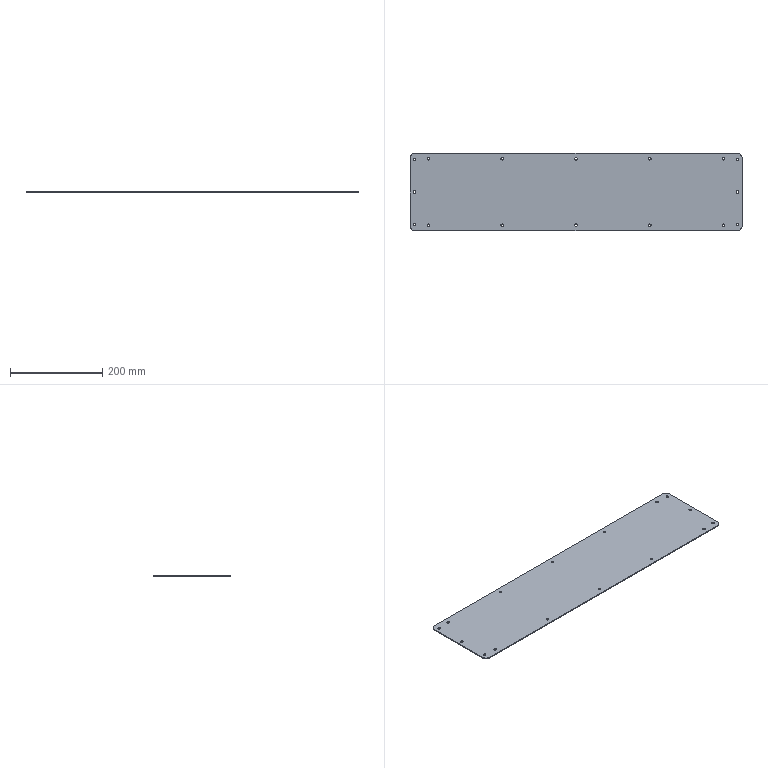Part | NX | features BREP 1 | 1 solid | 42 faces | box 720 x 168 x 2 mm | volume 240988 mm3 | cylinder 36 | plane 6 | commonest cylinder face diameters 5.5 x32 20 x4
STEP:
#1=CARTESIAN_POINT('',(352.75,0.,2.));
#2=VERTEX_POINT('',#1);
#3=CARTESIAN_POINT('',(347.25,0.,2.));
#4=VERTEX_POINT('',#3);
#5=CARTESIAN_POINT('',(350.,0.,2.));
#6=DIRECTION('',(0.,0.,-1.));
#7=DIRECTION('',(-1.,0.,0.));
#8=AXIS2_PLACEMENT_3D('',#5,#6,#7);
#9=CIRCLE('',#8,2.75);
#10=EDGE_CURVE('',#2,#4,#9,.T.);
#11=ORIENTED_EDGE('',*,*,#10,.F.);
#12=CARTESIAN_POINT('',(352.75,0.,0.));
#13=VERTEX_POINT('',#12);
#14=CARTESIAN_POINT('',(352.75,0.,0.));
#15=DIRECTION('',(0.,0.,-1.));
#16=VECTOR('',#15,1000.);
#17=LINE('',#14,#16);
#18=EDGE_CURVE('',#2,#13,#17,.T.);
#19=ORIENTED_EDGE('',*,*,#18,.T.);
#20=CARTESIAN_POINT('',(347.25,0.,0.));
#21=VERTEX_POINT('',#20);
#22=CARTESIAN_POINT('',(350.,0.,0.));
#23=DIRECTION('',(0.,0.,-1.));
#24=DIRECTION('',(-1.,0.,0.));
#25=AXIS2_PLACEMENT_3D('',#22,#23,#24);
#26=CIRCLE('',#25,2.75);
#27=EDGE_CURVE('',#13,#21,#26,.T.);
#28=ORIENTED_EDGE('',*,*,#27,.T.);
#29=CARTESIAN_POINT('',(347.25,0.,0.));
#30=DIRECTION('',(0.,0.,-1.));
#31=VECTOR('',#30,1000.);
#32=LINE('',#29,#31);
#33=EDGE_CURVE('',#4,#21,#32,.T.);
#34=ORIENTED_EDGE('',*,*,#33,.F.);
#35=EDGE_LOOP('',(#11,#19,#28,#34));
#36=FACE_BOUND('',#35,.T.);
#37=CARTESIAN_POINT('',(350.,0.,0.));
#38=DIRECTION('',(0.,0.,-1.));
#39=DIRECTION('',(-1.,0.,0.));
#40=AXIS2_PLACEMENT_3D('',#37,#38,#39);
#41=CYLINDRICAL_SURFACE('',#40,2.75);
#42=ADVANCED_FACE('',(#36),#41,.F.);
#43=CARTESIAN_POINT('',(352.75,70.,2.));
#44=VERTEX_POINT('',#43);
#45=CARTESIAN_POINT('',(347.25,70.,2.));
#46=VERTEX_POINT('',#45);
#47=CARTESIAN_POINT('',(350.,70.,2.));
#48=DIRECTION('',(0.,0.,-1.));
#49=DIRECTION('',(-1.,0.,0.));
#50=AXIS2_PLACEMENT_3D('',#47,#48,#49);
#51=CIRCLE('',#50,2.75);
#52=EDGE_CURVE('',#44,#46,#51,.T.);
#53=ORIENTED_EDGE('',*,*,#52,.F.);
#54=CARTESIAN_POINT('',(352.75,70.,0.));
#55=VERTEX_POINT('',#54);
#56=CARTESIAN_POINT('',(352.75,70.,0.));
#57=DIRECTION('',(0.,0.,-1.));
#58=VECTOR('',#57,1000.);
#59=LINE('',#56,#58);
#60=EDGE_CURVE('',#44,#55,#59,.T.);
#61=ORIENTED_EDGE('',*,*,#60,.T.);
#62=CARTESIAN_POINT('',(347.25,70.,0.));
#63=VERTEX_POINT('',#62);
#64=CARTESIAN_POINT('',(350.,70.,0.));
#65=DIRECTION('',(0.,0.,-1.));
#66=DIRECTION('',(-1.,0.,0.));
#67=AXIS2_PLACEMENT_3D('',#64,#65,#66);
#68=CIRCLE('',#67,2.75);
#69=EDGE_CURVE('',#55,#63,#68,.T.);
#70=ORIENTED_EDGE('',*,*,#69,.T.);
#71=CARTESIAN_POINT('',(347.25,70.,0.));
#72=DIRECTION('',(0.,0.,-1.));
#73=VECTOR('',#72,1000.);
#74=LINE('',#71,#73);
#75=EDGE_CURVE('',#46,#63,#74,.T.);
#76=ORIENTED_EDGE('',*,*,#75,.F.);
#77=EDGE_LOOP('',(#53,#61,#70,#76));
#78=FACE_BOUND('',#77,.T.);
#79=CARTESIAN_POINT('',(350.,70.,0.));
#80=DIRECTION('',(0.,0.,-1.));
#81=DIRECTION('',(-1.,0.,0.));
#82=AXIS2_PLACEMENT_3D('',#79,#80,#81);
#83=CYLINDRICAL_SURFACE('',#82,2.75);
#84=ADVANCED_FACE('',(#78),#83,.F.);
#85=CARTESIAN_POINT('',(352.75,-70.,2.));
#86=VERTEX_POINT('',#85);
#87=CARTESIAN_POINT('',(347.25,-70.,2.));
#88=VERTEX_POINT('',#87);
#89=CARTESIAN_POINT('',(350.,-70.,2.));
#90=DIRECTION('',(0.,0.,-1.));
#91=DIRECTION('',(-1.,0.,0.));
#92=AXIS2_PLACEMENT_3D('',#89,#90,#91);
#93=CIRCLE('',#92,2.75);
#94=EDGE_CURVE('',#86,#88,#93,.T.);
#95=ORIENTED_EDGE('',*,*,#94,.F.);
#96=CARTESIAN_POINT('',(352.75,-70.,0.));
#97=VERTEX_POINT('',#96);
#98=CARTESIAN_POINT('',(352.75,-70.,0.));
#99=DIRECTION('',(0.,0.,-1.));
#100=VECTOR('',#99,1000.);
#101=LINE('',#98,#100);
#102=EDGE_CURVE('',#86,#97,#101,.T.);
#103=ORIENTED_EDGE('',*,*,#102,.T.);
#104=CARTESIAN_POINT('',(347.25,-70.,0.));
#105=VERTEX_POINT('',#104);
#106=CARTESIAN_POINT('',(350.,-70.,0.));
#107=DIRECTION('',(0.,0.,-1.));
#108=DIRECTION('',(-1.,0.,0.));
#109=AXIS2_PLACEMENT_3D('',#106,#107,#108);
#110=CIRCLE('',#109,2.75);
#111=EDGE_CURVE('',#97,#105,#110,.T.);
#112=ORIENTED_EDGE('',*,*,#111,.T.);
#113=CARTESIAN_POINT('',(347.25,-70.,0.));
#114=DIRECTION('',(0.,0.,-1.));
#115=VECTOR('',#114,1000.);
#116=LINE('',#113,#115);
#117=EDGE_CURVE('',#88,#105,#116,.T.);
#118=ORIENTED_EDGE('',*,*,#117,.F.);
#119=EDGE_LOOP('',(#95,#103,#112,#118));
#120=FACE_BOUND('',#119,.T.);
#121=CARTESIAN_POINT('',(350.,-70.,0.));
#122=DIRECTION('',(0.,0.,-1.));
#123=DIRECTION('',(-1.,0.,0.));
#124=AXIS2_PLACEMENT_3D('',#121,#122,#123);
#125=CYLINDRICAL_SURFACE('',#124,2.75);
#126=ADVANCED_FACE('',(#120),#125,.F.);
#127=CARTESIAN_POINT('',(322.75,-72.,2.));
#128=VERTEX_POINT('',#127);
#129=CARTESIAN_POINT('',(317.25,-72.,2.));
#130=VERTEX_POINT('',#129);
#131=CARTESIAN_POINT('',(320.,-72.,2.));
#132=DIRECTION('',(0.,0.,-1.));
#133=DIRECTION('',(-1.,0.,0.));
#134=AXIS2_PLACEMENT_3D('',#131,#132,#133);
#135=CIRCLE('',#134,2.75);
#136=EDGE_CURVE('',#128,#130,#135,.T.);
#137=ORIENTED_EDGE('',*,*,#136,.F.);
#138=CARTESIAN_POINT('',(322.75,-72.,0.));
#139=VERTEX_POINT('',#138);
#140=CARTESIAN_POINT('',(322.75,-72.,0.));
#141=DIRECTION('',(0.,0.,-1.));
#142=VECTOR('',#141,1000.);
#143=LINE('',#140,#142);
#144=EDGE_CURVE('',#128,#139,#143,.T.);
#145=ORIENTED_EDGE('',*,*,#144,.T.);
#146=CARTESIAN_POINT('',(317.25,-72.,0.));
#147=VERTEX_POINT('',#146);
#148=CARTESIAN_POINT('',(320.,-72.,0.));
#149=DIRECTION('',(0.,0.,-1.));
#150=DIRECTION('',(-1.,0.,0.));
#151=AXIS2_PLACEMENT_3D('',#148,#149,#150);
#152=CIRCLE('',#151,2.75);
#153=EDGE_CURVE('',#139,#147,#152,.T.);
#154=ORIENTED_EDGE('',*,*,#153,.T.);
#155=CARTESIAN_POINT('',(317.25,-72.,0.));
#156=DIRECTION('',(0.,0.,-1.));
#157=VECTOR('',#156,1000.);
#158=LINE('',#155,#157);
#159=EDGE_CURVE('',#130,#147,#158,.T.);
#160=ORIENTED_EDGE('',*,*,#159,.F.);
#161=EDGE_LOOP('',(#137,#145,#154,#160));
#162=FACE_BOUND('',#161,.T.);
#163=CARTESIAN_POINT('',(320.,-72.,0.));
#164=DIRECTION('',(0.,0.,-1.));
#165=DIRECTION('',(-1.,0.,0.));
#166=AXIS2_PLACEMENT_3D('',#163,#164,#165);
#167=CYLINDRICAL_SURFACE('',#166,2.75);
#168=ADVANCED_FACE('',(#162),#167,.F.);
#169=CARTESIAN_POINT('',(2.75,-72.,2.));
#170=VERTEX_POINT('',#169);
#171=CARTESIAN_POINT('',(-2.75,-72.,2.));
#172=VERTEX_POINT('',#171);
#173=CARTESIAN_POINT('',(0.,-72.,2.));
#174=DIRECTION('',(0.,0.,-1.));
#175=DIRECTION('',(-1.,0.,0.));
#176=AXIS2_PLACEMENT_3D('',#173,#174,#175);
#177=CIRCLE('',#176,2.75);
#178=EDGE_CURVE('',#170,#172,#177,.T.);
#179=ORIENTED_EDGE('',*,*,#178,.F.);
#180=CARTESIAN_POINT('',(2.75,-72.,0.));
#181=VERTEX_POINT('',#180);
#182=CARTESIAN_POINT('',(2.75,-72.,0.));
#183=DIRECTION('',(0.,0.,-1.));
#184=VECTOR('',#183,1000.);
#185=LINE('',#182,#184);
#186=EDGE_CURVE('',#170,#181,#185,.T.);
#187=ORIENTED_EDGE('',*,*,#186,.T.);
#188=CARTESIAN_POINT('',(-2.75,-72.,0.));
#189=VERTEX_POINT('',#188);
#190=CARTESIAN_POINT('',(0.,-72.,0.));
#191=DIRECTION('',(0.,0.,-1.));
#192=DIRECTION('',(-1.,0.,0.));
#193=AXIS2_PLACEMENT_3D('',#190,#191,#192);
#194=CIRCLE('',#193,2.75);
#195=EDGE_CURVE('',#181,#189,#194,.T.);
#196=ORIENTED_EDGE('',*,*,#195,.T.);
#197=CARTESIAN_POINT('',(-2.75,-72.,0.));
#198=DIRECTION('',(0.,0.,-1.));
#199=VECTOR('',#198,1000.);
#200=LINE('',#197,#199);
#201=EDGE_CURVE('',#172,#189,#200,.T.);
#202=ORIENTED_EDGE('',*,*,#201,.F.);
#203=EDGE_LOOP('',(#179,#187,#196,#202));
#204=FACE_BOUND('',#203,.T.);
#205=CARTESIAN_POINT('',(0.,-72.,0.));
#206=DIRECTION('',(0.,0.,-1.));
#207=DIRECTION('',(-1.,0.,0.));
#208=AXIS2_PLACEMENT_3D('',#205,#206,#207);
#209=CYLINDRICAL_SURFACE('',#208,2.75);
#210=ADVANCED_FACE('',(#204),#209,.F.);
#211=CARTESIAN_POINT('',(162.75,-72.,2.));
#212=VERTEX_POINT('',#211);
#213=CARTESIAN_POINT('',(157.25,-72.,2.));
#214=VERTEX_POINT('',#213);
#215=CARTESIAN_POINT('',(160.,-72.,2.));
#216=DIRECTION('',(0.,0.,-1.));
#217=DIRECTION('',(-1.,0.,0.));
#218=AXIS2_PLACEMENT_3D('',#215,#216,#217);
#219=CIRCLE('',#218,2.75);
#220=EDGE_CURVE('',#212,#214,#219,.T.);
#221=ORIENTED_EDGE('',*,*,#220,.F.);
#222=CARTESIAN_POINT('',(162.75,-72.,0.));
#223=VERTEX_POINT('',#222);
#224=CARTESIAN_POINT('',(162.75,-72.,0.));
#225=DIRECTION('',(0.,0.,-1.));
#226=VECTOR('',#225,1000.);
#227=LINE('',#224,#226);
#228=EDGE_CURVE('',#212,#223,#227,.T.);
#229=ORIENTED_EDGE('',*,*,#228,.T.);
#230=CARTESIAN_POINT('',(157.25,-72.,0.));
#231=VERTEX_POINT('',#230);
#232=CARTESIAN_POINT('',(160.,-72.,0.));
#233=DIRECTION('',(0.,0.,-1.));
#234=DIRECTION('',(-1.,0.,0.));
#235=AXIS2_PLACEMENT_3D('',#232,#233,#234);
#236=CIRCLE('',#235,2.75);
#237=EDGE_CURVE('',#223,#231,#236,.T.);
#238=ORIENTED_EDGE('',*,*,#237,.T.);
#239=CARTESIAN_POINT('',(157.25,-72.,0.));
#240=DIRECTION('',(0.,0.,-1.));
#241=VECTOR('',#240,1000.);
#242=LINE('',#239,#241);
#243=EDGE_CURVE('',#214,#231,#242,.T.);
#244=ORIENTED_EDGE('',*,*,#243,.F.);
#245=EDGE_LOOP('',(#221,#229,#238,#244));
#246=FACE_BOUND('',#245,.T.);
#247=CARTESIAN_POINT('',(160.,-72.,0.));
#248=DIRECTION('',(0.,0.,-1.));
#249=DIRECTION('',(-1.,0.,0.));
#250=AXIS2_PLACEMENT_3D('',#247,#248,#249);
#251=CYLINDRICAL_SURFACE('',#250,2.75);
#252=ADVANCED_FACE('',(#246),#251,.F.);
#253=CARTESIAN_POINT('',(-157.25,-72.,2.));
#254=VERTEX_POINT('',#253);
#255=CARTESIAN_POINT('',(-162.75,-72.,2.));
#256=VERTEX_POINT('',#255);
#257=CARTESIAN_POINT('',(-160.,-72.,2.));
#258=DIRECTION('',(0.,0.,-1.));
#259=DIRECTION('',(-1.,0.,0.));
#260=AXIS2_PLACEMENT_3D('',#257,#258,#259);
#261=CIRCLE('',#260,2.75);
#262=EDGE_CURVE('',#254,#256,#261,.T.);
#263=ORIENTED_EDGE('',*,*,#262,.F.);
#264=CARTESIAN_POINT('',(-157.25,-72.,0.));
#265=VERTEX_POINT('',#264);
#266=CARTESIAN_POINT('',(-157.25,-72.,0.));
#267=DIRECTION('',(0.,0.,-1.));
#268=VECTOR('',#267,1000.);
#269=LINE('',#266,#268);
#270=EDGE_CURVE('',#254,#265,#269,.T.);
#271=ORIENTED_EDGE('',*,*,#270,.T.);
#272=CARTESIAN_POINT('',(-162.75,-72.,0.));
#273=VERTEX_POINT('',#272);
#274=CARTESIAN_POINT('',(-160.,-72.,0.));
#275=DIRECTION('',(0.,0.,-1.));
#276=DIRECTION('',(-1.,0.,0.));
#277=AXIS2_PLACEMENT_3D('',#274,#275,#276);
#278=CIRCLE('',#277,2.75);
#279=EDGE_CURVE('',#265,#273,#278,.T.);
#280=ORIENTED_EDGE('',*,*,#279,.T.);
#281=CARTESIAN_POINT('',(-162.75,-72.,0.));
#282=DIRECTION('',(0.,0.,-1.));
#283=VECTOR('',#282,1000.);
#284=LINE('',#281,#283);
#285=EDGE_CURVE('',#256,#273,#284,.T.);
#286=ORIENTED_EDGE('',*,*,#285,.F.);
#287=EDGE_LOOP('',(#263,#271,#280,#286));
#288=FACE_BOUND('',#287,.T.);
#289=CARTESIAN_POINT('',(-160.,-72.,0.));
#290=DIRECTION('',(0.,0.,-1.));
#291=DIRECTION('',(-1.,0.,0.));
#292=AXIS2_PLACEMENT_3D('',#289,#290,#291);
#293=CYLINDRICAL_SURFACE('',#292,2.75);
#294=ADVANCED_FACE('',(#288),#293,.F.);
#295=CARTESIAN_POINT('',(-317.25,-72.,2.));
#296=VERTEX_POINT('',#295);
#297=CARTESIAN_POINT('',(-322.75,-72.,2.));
#298=VERTEX_POINT('',#297);
#299=CARTESIAN_POINT('',(-320.,-72.,2.));
#300=DIRECTION('',(0.,0.,-1.));
#301=DIRECTION('',(-1.,0.,0.));
#302=AXIS2_PLACEMENT_3D('',#299,#300,#301);
#303=CIRCLE('',#302,2.75);
#304=EDGE_CURVE('',#296,#298,#303,.T.);
#305=ORIENTED_EDGE('',*,*,#304,.F.);
#306=CARTESIAN_POINT('',(-317.25,-72.,0.));
#307=VERTEX_POINT('',#306);
#308=CARTESIAN_POINT('',(-317.25,-72.,0.));
#309=DIRECTION('',(0.,0.,-1.));
#310=VECTOR('',#309,1000.);
#311=LINE('',#308,#310);
#312=EDGE_CURVE('',#296,#307,#311,.T.);
#313=ORIENTED_EDGE('',*,*,#312,.T.);
#314=CARTESIAN_POINT('',(-322.75,-72.,0.));
#315=VERTEX_POINT('',#314);
#316=CARTESIAN_POINT('',(-320.,-72.,0.));
#317=DIRECTION('',(0.,0.,-1.));
#318=DIRECTION('',(-1.,0.,0.));
#319=AXIS2_PLACEMENT_3D('',#316,#317,#318);
#320=CIRCLE('',#319,2.75);
#321=EDGE_CURVE('',#307,#315,#320,.T.);
#322=ORIENTED_EDGE('',*,*,#321,.T.);
#323=CARTESIAN_POINT('',(-322.75,-72.,0.));
#324=DIRECTION('',(0.,0.,-1.));
#325=VECTOR('',#324,1000.);
#326=LINE('',#323,#325);
#327=EDGE_CURVE('',#298,#315,#326,.T.);
#328=ORIENTED_EDGE('',*,*,#327,.F.);
#329=EDGE_LOOP('',(#305,#313,#322,#328));
#330=FACE_BOUND('',#329,.T.);
#331=CARTESIAN_POINT('',(-320.,-72.,0.));
#332=DIRECTION('',(0.,0.,-1.));
#333=DIRECTION('',(-1.,0.,0.));
#334=AXIS2_PLACEMENT_3D('',#331,#332,#333);
#335=CYLINDRICAL_SURFACE('',#334,2.75);
#336=ADVANCED_FACE('',(#330),#335,.F.);
#337=CARTESIAN_POINT('',(322.75,72.,2.));
#338=VERTEX_POINT('',#337);
#339=CARTESIAN_POINT('',(317.25,72.,2.));
#340=VERTEX_POINT('',#339);
#341=CARTESIAN_POINT('',(320.,72.,2.));
#342=DIRECTION('',(0.,0.,-1.));
#343=DIRECTION('',(-1.,0.,0.));
#344=AXIS2_PLACEMENT_3D('',#341,#342,#343);
#345=CIRCLE('',#344,2.75);
#346=EDGE_CURVE('',#338,#340,#345,.T.);
#347=ORIENTED_EDGE('',*,*,#346,.F.);
#348=CARTESIAN_POINT('',(322.75,72.,0.));
#349=VERTEX_POINT('',#348);
#350=CARTESIAN_POINT('',(322.75,72.,0.));
#351=DIRECTION('',(0.,0.,-1.));
#352=VECTOR('',#351,1000.);
#353=LINE('',#350,#352);
#354=EDGE_CURVE('',#338,#349,#353,.T.);
#355=ORIENTED_EDGE('',*,*,#354,.T.);
#356=CARTESIAN_POINT('',(317.25,72.,0.));
#357=VERTEX_POINT('',#356);
#358=CARTESIAN_POINT('',(320.,72.,0.));
#359=DIRECTION('',(0.,0.,-1.));
#360=DIRECTION('',(-1.,0.,0.));
#361=AXIS2_PLACEMENT_3D('',#358,#359,#360);
#362=CIRCLE('',#361,2.75);
#363=EDGE_CURVE('',#349,#357,#362,.T.);
#364=ORIENTED_EDGE('',*,*,#363,.T.);
#365=CARTESIAN_POINT('',(317.25,72.,0.));
#366=DIRECTION('',(0.,0.,-1.));
#367=VECTOR('',#366,1000.);
#368=LINE('',#365,#367);
#369=EDGE_CURVE('',#340,#357,#368,.T.);
#370=ORIENTED_EDGE('',*,*,#369,.F.);
#371=EDGE_LOOP('',(#347,#355,#364,#370));
#372=FACE_BOUND('',#371,.T.);
#373=CARTESIAN_POINT('',(320.,72.,0.));
#374=DIRECTION('',(0.,0.,-1.));
#375=DIRECTION('',(-1.,0.,0.));
#376=AXIS2_PLACEMENT_3D('',#373,#374,#375);
#377=CYLINDRICAL_SURFACE('',#376,2.75);
#378=ADVANCED_FACE('',(#372),#377,.F.);
#379=CARTESIAN_POINT('',(2.75,72.,2.));
#380=VERTEX_POINT('',#379);
#381=CARTESIAN_POINT('',(-2.75,72.,2.));
#382=VERTEX_POINT('',#381);
#383=CARTESIAN_POINT('',(0.,72.,2.));
#384=DIRECTION('',(0.,0.,-1.));
#385=DIRECTION('',(-1.,0.,0.));
#386=AXIS2_PLACEMENT_3D('',#383,#384,#385);
#387=CIRCLE('',#386,2.75);
#388=EDGE_CURVE('',#380,#382,#387,.T.);
#389=ORIENTED_EDGE('',*,*,#388,.F.);
#390=CARTESIAN_POINT('',(2.75,72.,0.));
#391=VERTEX_POINT('',#390);
#392=CARTESIAN_POINT('',(2.75,72.,0.));
#393=DIRECTION('',(0.,0.,-1.));
#394=VECTOR('',#393,1000.);
#395=LINE('',#392,#394);
#396=EDGE_CURVE('',#380,#391,#395,.T.);
#397=ORIENTED_EDGE('',*,*,#396,.T.);
#398=CARTESIAN_POINT('',(-2.75,72.,0.));
#399=VERTEX_POINT('',#398);
#400=CARTESIAN_POINT('',(0.,72.,0.));
#401=DIRECTION('',(0.,0.,-1.));
#402=DIRECTION('',(-1.,0.,0.));
#403=AXIS2_PLACEMENT_3D('',#400,#401,#402);
#404=CIRCLE('',#403,2.75);
#405=EDGE_CURVE('',#391,#399,#404,.T.);
#406=ORIENTED_EDGE('',*,*,#405,.T.);
#407=CARTESIAN_POINT('',(-2.75,72.,0.));
#408=DIRECTION('',(0.,0.,-1.));
#409=VECTOR('',#408,1000.);
#410=LINE('',#407,#409);
#411=EDGE_CURVE('',#382,#399,#410,.T.);
#412=ORIENTED_EDGE('',*,*,#411,.F.);
#413=EDGE_LOOP('',(#389,#397,#406,#412));
#414=FACE_BOUND('',#413,.T.);
#415=CARTESIAN_POINT('',(0.,72.,0.));
#416=DIRECTION('',(0.,0.,-1.));
#417=DIRECTION('',(-1.,0.,0.));
#418=AXIS2_PLACEMENT_3D('',#415,#416,#417);
#419=CYLINDRICAL_SURFACE('',#418,2.75);
#420=ADVANCED_FACE('',(#414),#419,.F.);
#421=CARTESIAN_POINT('',(162.75,72.,2.));
#422=VERTEX_POINT('',#421);
#423=CARTESIAN_POINT('',(157.25,72.,2.));
#424=VERTEX_POINT('',#423);
#425=CARTESIAN_POINT('',(160.,72.,2.));
#426=DIRECTION('',(0.,0.,-1.));
#427=DIRECTION('',(-1.,0.,0.));
#428=AXIS2_PLACEMENT_3D('',#425,#426,#427);
#429=CIRCLE('',#428,2.75);
#430=EDGE_CURVE('',#422,#424,#429,.T.);
#431=ORIENTED_EDGE('',*,*,#430,.F.);
#432=CARTESIAN_POINT('',(162.75,72.,0.));
#433=VERTEX_POINT('',#432);
#434=CARTESIAN_POINT('',(162.75,72.,0.));
#435=DIRECTION('',(0.,0.,-1.));
#436=VECTOR('',#435,1000.);
#437=LINE('',#434,#436);
#438=EDGE_CURVE('',#422,#433,#437,.T.);
#439=ORIENTED_EDGE('',*,*,#438,.T.);
#440=CARTESIAN_POINT('',(157.25,72.,0.));
#441=VERTEX_POINT('',#440);
#442=CARTESIAN_POINT('',(160.,72.,0.));
#443=DIRECTION('',(0.,0.,-1.));
#444=DIRECTION('',(-1.,0.,0.));
#445=AXIS2_PLACEMENT_3D('',#442,#443,#444);
#446=CIRCLE('',#445,2.75);
#447=EDGE_CURVE('',#433,#441,#446,.T.);
#448=ORIENTED_EDGE('',*,*,#447,.T.);
#449=CARTESIAN_POINT('',(157.25,72.,0.));
#450=DIRECTION('',(0.,0.,-1.));
#451=VECTOR('',#450,1000.);
#452=LINE('',#449,#451);
#453=EDGE_CURVE('',#424,#441,#452,.T.);
#454=ORIENTED_EDGE('',*,*,#453,.F.);
#455=EDGE_LOOP('',(#431,#439,#448,#454));
#456=FACE_BOUND('',#455,.T.);
#457=CARTESIAN_POINT('',(160.,72.,0.));
#458=DIRECTION('',(0.,0.,-1.));
#459=DIRECTION('',(-1.,0.,0.));
#460=AXIS2_PLACEMENT_3D('',#457,#458,#459);
#461=CYLINDRICAL_SURFACE('',#460,2.75);
#462=ADVANCED_FACE('',(#456),#461,.F.);
#463=CARTESIAN_POINT('',(-157.25,72.,2.));
#464=VERTEX_POINT('',#463);
#465=CARTESIAN_POINT('',(-162.75,72.,2.));
#466=VERTEX_POINT('',#465);
#467=CARTESIAN_POINT('',(-160.,72.,2.));
#468=DIRECTION('',(0.,0.,-1.));
#469=DIRECTION('',(-1.,0.,0.));
#470=AXIS2_PLACEMENT_3D('',#467,#468,#469);
#471=CIRCLE('',#470,2.75);
#472=EDGE_CURVE('',#464,#466,#471,.T.);
#473=ORIENTED_EDGE('',*,*,#472,.F.);
#474=CARTESIAN_POINT('',(-157.25,72.,0.));
#475=VERTEX_POINT('',#474);
#476=CARTESIAN_POINT('',(-157.25,72.,0.));
#477=DIRECTION('',(0.,0.,-1.));
#478=VECTOR('',#477,1000.);
#479=LINE('',#476,#478);
#480=EDGE_CURVE('',#464,#475,#479,.T.);
#481=ORIENTED_EDGE('',*,*,#480,.T.);
#482=CARTESIAN_POINT('',(-162.75,72.,0.));
#483=VERTEX_POINT('',#482);
#484=CARTESIAN_POINT('',(-160.,72.,0.));
#485=DIRECTION('',(0.,0.,-1.));
#486=DIRECTION('',(-1.,0.,0.));
#487=AXIS2_PLACEMENT_3D('',#484,#485,#486);
#488=CIRCLE('',#487,2.75);
#489=EDGE_CURVE('',#475,#483,#488,.T.);
#490=ORIENTED_EDGE('',*,*,#489,.T.);
#491=CARTESIAN_POINT('',(-162.75,72.,0.));
#492=DIRECTION('',(0.,0.,-1.));
#493=VECTOR('',#492,1000.);
#494=LINE('',#491,#493);
#495=EDGE_CURVE('',#466,#483,#494,.T.);
#496=ORIENTED_EDGE('',*,*,#495,.F.);
#497=EDGE_LOOP('',(#473,#481,#490,#496));
#498=FACE_BOUND('',#497,.T.);
#499=CARTESIAN_POINT('',(-160.,72.,0.));
#500=DIRECTION('',(0.,0.,-1.));
#501=DIRECTION('',(-1.,0.,0.));
#502=AXIS2_PLACEMENT_3D('',#499,#500,#501);
#503=CYLINDRICAL_SURFACE('',#502,2.75);
#504=ADVANCED_FACE('',(#498),#503,.F.);
#505=CARTESIAN_POINT('',(-317.25,72.,2.));
#506=VERTEX_POINT('',#505);
#507=CARTESIAN_POINT('',(-322.75,72.,2.));
#508=VERTEX_POINT('',#507);
#509=CARTESIAN_POINT('',(-320.,72.,2.));
#510=DIRECTION('',(0.,0.,-1.));
#511=DIRECTION('',(-1.,0.,0.));
#512=AXIS2_PLACEMENT_3D('',#509,#510,#511);
#513=CIRCLE('',#512,2.75);
#514=EDGE_CURVE('',#506,#508,#513,.T.);
#515=ORIENTED_EDGE('',*,*,#514,.F.);
#516=CARTESIAN_POINT('',(-317.25,72.,0.));
#517=VERTEX_POINT('',#516);
#518=CARTESIAN_POINT('',(-317.25,72.,0.));
#519=DIRECTION('',(0.,0.,-1.));
#520=VECTOR('',#519,1000.);
#521=LINE('',#518,#520);
#522=EDGE_CURVE('',#506,#517,#521,.T.);
#523=ORIENTED_EDGE('',*,*,#522,.T.);
#524=CARTESIAN_POINT('',(-322.75,72.,0.));
#525=VERTEX_POINT('',#524);
#526=CARTESIAN_POINT('',(-320.,72.,0.));
#527=DIRECTION('',(0.,0.,-1.));
#528=DIRECTION('',(-1.,0.,0.));
#529=AXIS2_PLACEMENT_3D('',#526,#527,#528);
#530=CIRCLE('',#529,2.75);
#531=EDGE_CURVE('',#517,#525,#530,.T.);
#532=ORIENTED_EDGE('',*,*,#531,.T.);
#533=CARTESIAN_POINT('',(-322.75,72.,0.));
#534=DIRECTION('',(0.,0.,-1.));
#535=VECTOR('',#534,1000.);
#536=LINE('',#533,#535);
#537=EDGE_CURVE('',#508,#525,#536,.T.);
#538=ORIENTED_EDGE('',*,*,#537,.F.);
#539=EDGE_LOOP('',(#515,#523,#532,#538));
#540=FACE_BOUND('',#539,.T.);
#541=CARTESIAN_POINT('',(-320.,72.,0.));
#542=DIRECTION('',(0.,0.,-1.));
#543=DIRECTION('',(-1.,0.,0.));
#544=AXIS2_PLACEMENT_3D('',#541,#542,#543);
#545=CYLINDRICAL_SURFACE('',#544,2.75);
#546=ADVANCED_FACE('',(#540),#545,.F.);
#547=CARTESIAN_POINT('',(-347.25,0.,2.));
#548=VERTEX_POINT('',#547);
#549=CARTESIAN_POINT('',(-352.75,0.,2.));
#550=VERTEX_POINT('',#549);
#551=CARTESIAN_POINT('',(-350.,0.,2.));
#552=DIRECTION('',(0.,0.,-1.));
#553=DIRECTION('',(-1.,0.,0.));
#554=AXIS2_PLACEMENT_3D('',#551,#552,#553);
#555=CIRCLE('',#554,2.75);
#556=EDGE_CURVE('',#548,#550,#555,.T.);
#557=ORIENTED_EDGE('',*,*,#556,.F.);
#558=CARTESIAN_POINT('',(-347.25,0.,0.));
#559=VERTEX_POINT('',#558);
#560=CARTESIAN_POINT('',(-347.25,0.,0.));
#561=DIRECTION('',(0.,0.,-1.));
#562=VECTOR('',#561,1000.);
#563=LINE('',#560,#562);
#564=EDGE_CURVE('',#548,#559,#563,.T.);
#565=ORIENTED_EDGE('',*,*,#564,.T.);
#566=CARTESIAN_POINT('',(-352.75,0.,0.));
#567=VERTEX_POINT('',#566);
#568=CARTESIAN_POINT('',(-350.,0.,0.));
#569=DIRECTION('',(0.,0.,-1.));
#570=DIRECTION('',(-1.,0.,0.));
#571=AXIS2_PLACEMENT_3D('',#568,#569,#570);
#572=CIRCLE('',#571,2.75);
#573=EDGE_CURVE('',#559,#567,#572,.T.);
#574=ORIENTED_EDGE('',*,*,#573,.T.);
#575=CARTESIAN_POINT('',(-352.75,0.,0.));
#576=DIRECTION('',(0.,0.,-1.));
#577=VECTOR('',#576,1000.);
#578=LINE('',#575,#577);
#579=EDGE_CURVE('',#550,#567,#578,.T.);
#580=ORIENTED_EDGE('',*,*,#579,.F.);
#581=EDGE_LOOP('',(#557,#565,#574,#580));
#582=FACE_BOUND('',#581,.T.);
#583=CARTESIAN_POINT('',(-350.,0.,0.));
#584=DIRECTION('',(0.,0.,-1.));
#585=DIRECTION('',(-1.,0.,0.));
#586=AXIS2_PLACEMENT_3D('',#583,#584,#585);
#587=CYLINDRICAL_SURFACE('',#586,2.75);
#588=ADVANCED_FACE('',(#582),#587,.F.);
#589=CARTESIAN_POINT('',(-347.25,70.,2.));
#590=VERTEX_POINT('',#589);
#591=CARTESIAN_POINT('',(-352.75,70.,2.));
#592=VERTEX_POINT('',#591);
#593=CARTESIAN_POINT('',(-350.,70.,2.));
#594=DIRECTION('',(0.,0.,-1.));
#595=DIRECTION('',(-1.,0.,0.));
#596=AXIS2_PLACEMENT_3D('',#593,#594,#595);
#597=CIRCLE('',#596,2.75);
#598=EDGE_CURVE('',#590,#592,#597,.T.);
#599=ORIENTED_EDGE('',*,*,#598,.F.);
#600=CARTESIAN_POINT('',(-347.25,70.,0.));
#601=VERTEX_POINT('',#600);
#602=CARTESIAN_POINT('',(-347.25,70.,0.));
#603=DIRECTION('',(0.,0.,-1.));
#604=VECTOR('',#603,1000.);
#605=LINE('',#602,#604);
#606=EDGE_CURVE('',#590,#601,#605,.T.);
#607=ORIENTED_EDGE('',*,*,#606,.T.);
#608=CARTESIAN_POINT('',(-352.75,70.,0.));
#609=VERTEX_POINT('',#608);
#610=CARTESIAN_POINT('',(-350.,70.,0.));
#611=DIRECTION('',(0.,0.,-1.));
#612=DIRECTION('',(-1.,0.,0.));
#613=AXIS2_PLACEMENT_3D('',#610,#611,#612);
#614=CIRCLE('',#613,2.75);
#615=EDGE_CURVE('',#601,#609,#614,.T.);
#616=ORIENTED_EDGE('',*,*,#615,.T.);
#617=CARTESIAN_POINT('',(-352.75,70.,0.));
#618=DIRECTION('',(0.,0.,-1.));
#619=VECTOR('',#618,1000.);
#620=LINE('',#617,#619);
#621=EDGE_CURVE('',#592,#609,#620,.T.);
#622=ORIENTED_EDGE('',*,*,#621,.F.);
#623=EDGE_LOOP('',(#599,#607,#616,#622));
#624=FACE_BOUND('',#623,.T.);
#625=CARTESIAN_POINT('',(-350.,70.,0.));
#626=DIRECTION('',(0.,0.,-1.));
#627=DIRECTION('',(-1.,0.,0.));
#628=AXIS2_PLACEMENT_3D('',#625,#626,#627);
#629=CYLINDRICAL_SURFACE('',#628,2.75);
#630=ADVANCED_FACE('',(#624),#629,.F.);
#631=CARTESIAN_POINT('',(-347.25,-70.,2.));
#632=VERTEX_POINT('',#631);
#633=CARTESIAN_POINT('',(-352.75,-70.,2.));
#634=VERTEX_POINT('',#633);
#635=CARTESIAN_POINT('',(-350.,-70.,2.));
#636=DIRECTION('',(0.,0.,-1.));
#637=DIRECTION('',(-1.,0.,0.));
#638=AXIS2_PLACEMENT_3D('',#635,#636,#637);
#639=CIRCLE('',#638,2.75);
#640=EDGE_CURVE('',#632,#634,#639,.T.);
#641=ORIENTED_EDGE('',*,*,#640,.F.);
#642=CARTESIAN_POINT('',(-347.25,-70.,0.));
#643=VERTEX_POINT('',#642);
#644=CARTESIAN_POINT('',(-347.25,-70.,0.));
#645=DIRECTION('',(0.,0.,-1.));
#646=VECTOR('',#645,1000.);
#647=LINE('',#644,#646);
#648=EDGE_CURVE('',#632,#643,#647,.T.);
#649=ORIENTED_EDGE('',*,*,#648,.T.);
#650=CARTESIAN_POINT('',(-352.75,-70.,0.));
#651=VERTEX_POINT('',#650);
#652=CARTESIAN_POINT('',(-350.,-70.,0.));
#653=DIRECTION('',(0.,0.,-1.));
#654=DIRECTION('',(-1.,0.,0.));
#655=AXIS2_PLACEMENT_3D('',#652,#653,#654);
#656=CIRCLE('',#655,2.75);
#657=EDGE_CURVE('',#643,#651,#656,.T.);
#658=ORIENTED_EDGE('',*,*,#657,.T.);
#659=CARTESIAN_POINT('',(-352.75,-70.,0.));
#660=DIRECTION('',(0.,0.,-1.));
#661=VECTOR('',#660,1000.);
#662=LINE('',#659,#661);
#663=EDGE_CURVE('',#634,#651,#662,.T.);
#664=ORIENTED_EDGE('',*,*,#663,.F.);
#665=EDGE_LOOP('',(#641,#649,#658,#664));
#666=FACE_BOUND('',#665,.T.);
#667=CARTESIAN_POINT('',(-350.,-70.,0.));
#668=DIRECTION('',(0.,0.,-1.));
#669=DIRECTION('',(-1.,0.,0.));
#670=AXIS2_PLACEMENT_3D('',#667,#668,#669);
#671=CYLINDRICAL_SURFACE('',#670,2.75);
#672=ADVANCED_FACE('',(#666),#671,.F.);
#673=CARTESIAN_POINT('',(-360.,74.,2.));
#674=VERTEX_POINT('',#673);
#675=CARTESIAN_POINT('',(-360.,-74.,2.));
#676=VERTEX_POINT('',#675);
#677=CARTESIAN_POINT('',(-360.,-84.,2.));
#678=DIRECTION('',(0.,-1.,0.));
#679=VECTOR('',#678,1000.);
#680=LINE('',#677,#679);
#681=EDGE_CURVE('',#674,#676,#680,.T.);
#682=ORIENTED_EDGE('',*,*,#681,.F.);
#683=CARTESIAN_POINT('',(-360.,74.,0.));
#684=VERTEX_POINT('',#683);
#685=CARTESIAN_POINT('',(-360.,74.,2.));
#686=DIRECTION('',(0.,0.,-1.));
#687=VECTOR('',#686,1000.);
#688=LINE('',#685,#687);
#689=EDGE_CURVE('',#674,#684,#688,.T.);
#690=ORIENTED_EDGE('',*,*,#689,.T.);
#691=CARTESIAN_POINT('',(-360.,-74.,0.));
#692=VERTEX_POINT('',#691);
#693=CARTESIAN_POINT('',(-360.,-84.,0.));
#694=DIRECTION('',(0.,-1.,0.));
#695=VECTOR('',#694,1000.);
#696=LINE('',#693,#695);
#697=EDGE_CURVE('',#684,#692,#696,.T.);
#698=ORIENTED_EDGE('',*,*,#697,.T.);
#699=CARTESIAN_POINT('',(-360.,-74.,2.));
#700=DIRECTION('',(0.,0.,1.));
#701=VECTOR('',#700,1000.);
#702=LINE('',#699,#701);
#703=EDGE_CURVE('',#692,#676,#702,.T.);
#704=ORIENTED_EDGE('',*,*,#703,.T.);
#705=EDGE_LOOP('',(#682,#690,#698,#704));
#706=FACE_BOUND('',#705,.T.);
#707=CARTESIAN_POINT('',(-360.,-84.,2.));
#708=DIRECTION('',(1.,0.,0.));
#709=DIRECTION('',(0.,1.,0.));
#710=AXIS2_PLACEMENT_3D('',#707,#708,#709);
#711=PLANE('',#710);
#712=ADVANCED_FACE('',(#706),#711,.F.);
#713=CARTESIAN_POINT('',(-350.,-84.,2.));
#714=VERTEX_POINT('',#713);
#715=CARTESIAN_POINT('',(350.,-84.,2.));
#716=VERTEX_POINT('',#715);
#717=CARTESIAN_POINT('',(360.,-84.,2.));
#718=DIRECTION('',(1.,0.,0.));
#719=VECTOR('',#718,1000.);
#720=LINE('',#717,#719);
#721=EDGE_CURVE('',#714,#716,#720,.T.);
#722=ORIENTED_EDGE('',*,*,#721,.F.);
#723=CARTESIAN_POINT('',(-350.,-84.,0.));
#724=VERTEX_POINT('',#723);
#725=CARTESIAN_POINT('',(-350.,-84.,2.));
#726=DIRECTION('',(0.,0.,-1.));
#727=VECTOR('',#726,1000.);
#728=LINE('',#725,#727);
#729=EDGE_CURVE('',#714,#724,#728,.T.);
#730=ORIENTED_EDGE('',*,*,#729,.T.);
#731=CARTESIAN_POINT('',(350.,-84.,0.));
#732=VERTEX_POINT('',#731);
#733=CARTESIAN_POINT('',(360.,-84.,0.));
#734=DIRECTION('',(1.,0.,0.));
#735=VECTOR('',#734,1000.);
#736=LINE('',#733,#735);
#737=EDGE_CURVE('',#724,#732,#736,.T.);
#738=ORIENTED_EDGE('',*,*,#737,.T.);
#739=CARTESIAN_POINT('',(350.,-84.,2.));
#740=DIRECTION('',(0.,0.,1.));
#741=VECTOR('',#740,1000.);
#742=LINE('',#739,#741);
#743=EDGE_CURVE('',#732,#716,#742,.T.);
#744=ORIENTED_EDGE('',*,*,#743,.T.);
#745=EDGE_LOOP('',(#722,#730,#738,#744));
#746=FACE_BOUND('',#745,.T.);
#747=CARTESIAN_POINT('',(360.,-84.,2.));
#748=DIRECTION('',(0.,1.,0.));
#749=DIRECTION('',(1.,0.,0.));
#750=AXIS2_PLACEMENT_3D('',#747,#748,#749);
#751=PLANE('',#750);
#752=ADVANCED_FACE('',(#746),#751,.F.);
#753=CARTESIAN_POINT('',(360.,-74.,2.));
#754=VERTEX_POINT('',#753);
#755=CARTESIAN_POINT('',(360.,74.,2.));
#756=VERTEX_POINT('',#755);
#757=CARTESIAN_POINT('',(360.,-84.,2.));
#758=DIRECTION('',(0.,1.,0.));
#759=VECTOR('',#758,1000.);
#760=LINE('',#757,#759);
#761=EDGE_CURVE('',#754,#756,#760,.T.);
#762=ORIENTED_EDGE('',*,*,#761,.F.);
#763=CARTESIAN_POINT('',(360.,-74.,0.));
#764=VERTEX_POINT('',#763);
#765=CARTESIAN_POINT('',(360.,-74.,2.));
#766=DIRECTION('',(0.,0.,-1.));
#767=VECTOR('',#766,1000.);
#768=LINE('',#765,#767);
#769=EDGE_CURVE('',#754,#764,#768,.T.);
#770=ORIENTED_EDGE('',*,*,#769,.T.);
#771=CARTESIAN_POINT('',(360.,74.,0.));
#772=VERTEX_POINT('',#771);
#773=CARTESIAN_POINT('',(360.,-84.,0.));
#774=DIRECTION('',(0.,1.,0.));
#775=VECTOR('',#774,1000.);
#776=LINE('',#773,#775);
#777=EDGE_CURVE('',#764,#772,#776,.T.);
#778=ORIENTED_EDGE('',*,*,#777,.T.);
#779=CARTESIAN_POINT('',(360.,74.,2.));
#780=DIRECTION('',(0.,0.,1.));
#781=VECTOR('',#780,1000.);
#782=LINE('',#779,#781);
#783=EDGE_CURVE('',#772,#756,#782,.T.);
#784=ORIENTED_EDGE('',*,*,#783,.T.);
#785=EDGE_LOOP('',(#762,#770,#778,#784));
#786=FACE_BOUND('',#785,.T.);
#787=CARTESIAN_POINT('',(360.,-84.,2.));
#788=DIRECTION('',(-1.,0.,0.));
#789=DIRECTION('',(0.,0.,1.));
#790=AXIS2_PLACEMENT_3D('',#787,#788,#789);
#791=PLANE('',#790);
#792=ADVANCED_FACE('',(#786),#791,.F.);
#793=CARTESIAN_POINT('',(350.,84.,0.));
#794=VERTEX_POINT('',#793);
#795=CARTESIAN_POINT('',(-350.,84.,0.));
#796=VERTEX_POINT('',#795);
#797=CARTESIAN_POINT('',(360.,84.,0.));
#798=DIRECTION('',(-1.,0.,0.));
#799=VECTOR('',#798,1000.);
#800=LINE('',#797,#799);
#801=EDGE_CURVE('',#794,#796,#800,.T.);
#802=ORIENTED_EDGE('',*,*,#801,.T.);
#803=CARTESIAN_POINT('',(-350.,84.,2.));
#804=VERTEX_POINT('',#803);
#805=CARTESIAN_POINT('',(-350.,84.,2.));
#806=DIRECTION('',(0.,0.,1.));
#807=VECTOR('',#806,1000.);
#808=LINE('',#805,#807);
#809=EDGE_CURVE('',#796,#804,#808,.T.);
#810=ORIENTED_EDGE('',*,*,#809,.T.);
#811=CARTESIAN_POINT('',(350.,84.,2.));
#812=VERTEX_POINT('',#811);
#813=CARTESIAN_POINT('',(360.,84.,2.));
#814=DIRECTION('',(-1.,0.,0.));
#815=VECTOR('',#814,1000.);
#816=LINE('',#813,#815);
#817=EDGE_CURVE('',#812,#804,#816,.T.);
#818=ORIENTED_EDGE('',*,*,#817,.F.);
#819=CARTESIAN_POINT('',(350.,84.,2.));
#820=DIRECTION('',(0.,0.,-1.));
#821=VECTOR('',#820,1000.);
#822=LINE('',#819,#821);
#823=EDGE_CURVE('',#812,#794,#822,.T.);
#824=ORIENTED_EDGE('',*,*,#823,.T.);
#825=EDGE_LOOP('',(#802,#810,#818,#824));
#826=FACE_BOUND('',#825,.T.);
#827=CARTESIAN_POINT('',(360.,84.,2.));
#828=DIRECTION('',(0.,-1.,0.));
#829=DIRECTION('',(0.,0.,-1.));
#830=AXIS2_PLACEMENT_3D('',#827,#828,#829);
#831=PLANE('',#830);
#832=ADVANCED_FACE('',(#826),#831,.F.);
#833=ORIENTED_EDGE('',*,*,#817,.T.);
#834=CARTESIAN_POINT('',(-350.,74.,2.));
#835=DIRECTION('',(0.,0.,1.));
#836=DIRECTION('',(1.,0.,0.));
#837=AXIS2_PLACEMENT_3D('',#834,#835,#836);
#838=CIRCLE('',#837,10.);
#839=EDGE_CURVE('',#804,#674,#838,.T.);
#840=ORIENTED_EDGE('',*,*,#839,.T.);
#841=ORIENTED_EDGE('',*,*,#681,.T.);
#842=CARTESIAN_POINT('',(-350.,-74.,2.));
#843=DIRECTION('',(0.,0.,1.));
#844=DIRECTION('',(1.,0.,0.));
#845=AXIS2_PLACEMENT_3D('',#842,#843,#844);
#846=CIRCLE('',#845,10.);
#847=EDGE_CURVE('',#676,#714,#846,.T.);
#848=ORIENTED_EDGE('',*,*,#847,.T.);
#849=ORIENTED_EDGE('',*,*,#721,.T.);
#850=CARTESIAN_POINT('',(350.,-74.,2.));
#851=DIRECTION('',(0.,0.,1.));
#852=DIRECTION('',(1.,0.,0.));
#853=AXIS2_PLACEMENT_3D('',#850,#851,#852);
#854=CIRCLE('',#853,10.);
#855=EDGE_CURVE('',#716,#754,#854,.T.);
#856=ORIENTED_EDGE('',*,*,#855,.T.);
#857=ORIENTED_EDGE('',*,*,#761,.T.);
#858=CARTESIAN_POINT('',(350.,74.,2.));
#859=DIRECTION('',(0.,0.,1.));
#860=DIRECTION('',(1.,0.,0.));
#861=AXIS2_PLACEMENT_3D('',#858,#859,#860);
#862=CIRCLE('',#861,10.);
#863=EDGE_CURVE('',#756,#812,#862,.T.);
#864=ORIENTED_EDGE('',*,*,#863,.T.);
#865=EDGE_LOOP('',(#833,#840,#841,#848,#849,#856,#857,#864));
#866=FACE_BOUND('',#865,.T.);
#867=CARTESIAN_POINT('',(350.,0.,2.));
#868=DIRECTION('',(0.,0.,-1.));
#869=DIRECTION('',(-1.,0.,0.));
#870=AXIS2_PLACEMENT_3D('',#867,#868,#869);
#871=CIRCLE('',#870,2.75);
#872=EDGE_CURVE('',#4,#2,#871,.T.);
#873=ORIENTED_EDGE('',*,*,#872,.T.);
#874=ORIENTED_EDGE('',*,*,#10,.T.);
#875=EDGE_LOOP('',(#873,#874));
#876=FACE_BOUND('',#875,.T.);
#877=CARTESIAN_POINT('',(350.,70.,2.));
#878=DIRECTION('',(0.,0.,-1.));
#879=DIRECTION('',(-1.,0.,0.));
#880=AXIS2_PLACEMENT_3D('',#877,#878,#879);
#881=CIRCLE('',#880,2.75);
#882=EDGE_CURVE('',#46,#44,#881,.T.);
#883=ORIENTED_EDGE('',*,*,#882,.T.);
#884=ORIENTED_EDGE('',*,*,#52,.T.);
#885=EDGE_LOOP('',(#883,#884));
#886=FACE_BOUND('',#885,.T.);
#887=CARTESIAN_POINT('',(350.,-70.,2.));
#888=DIRECTION('',(0.,0.,-1.));
#889=DIRECTION('',(-1.,0.,0.));
#890=AXIS2_PLACEMENT_3D('',#887,#888,#889);
#891=CIRCLE('',#890,2.75);
#892=EDGE_CURVE('',#88,#86,#891,.T.);
#893=ORIENTED_EDGE('',*,*,#892,.T.);
#894=ORIENTED_EDGE('',*,*,#94,.T.);
#895=EDGE_LOOP('',(#893,#894));
#896=FACE_BOUND('',#895,.T.);
#897=CARTESIAN_POINT('',(320.,-72.,2.));
#898=DIRECTION('',(0.,0.,-1.));
#899=DIRECTION('',(-1.,0.,0.));
#900=AXIS2_PLACEMENT_3D('',#897,#898,#899);
#901=CIRCLE('',#900,2.75);
#902=EDGE_CURVE('',#130,#128,#901,.T.);
#903=ORIENTED_EDGE('',*,*,#902,.T.);
#904=ORIENTED_EDGE('',*,*,#136,.T.);
#905=EDGE_LOOP('',(#903,#904));
#906=FACE_BOUND('',#905,.T.);
#907=CARTESIAN_POINT('',(0.,-72.,2.));
#908=DIRECTION('',(0.,0.,-1.));
#909=DIRECTION('',(-1.,0.,0.));
#910=AXIS2_PLACEMENT_3D('',#907,#908,#909);
#911=CIRCLE('',#910,2.75);
#912=EDGE_CURVE('',#172,#170,#911,.T.);
#913=ORIENTED_EDGE('',*,*,#912,.T.);
#914=ORIENTED_EDGE('',*,*,#178,.T.);
#915=EDGE_LOOP('',(#913,#914));
#916=FACE_BOUND('',#915,.T.);
#917=CARTESIAN_POINT('',(160.,-72.,2.));
#918=DIRECTION('',(0.,0.,-1.));
#919=DIRECTION('',(-1.,0.,0.));
#920=AXIS2_PLACEMENT_3D('',#917,#918,#919);
#921=CIRCLE('',#920,2.75);
#922=EDGE_CURVE('',#214,#212,#921,.T.);
#923=ORIENTED_EDGE('',*,*,#922,.T.);
#924=ORIENTED_EDGE('',*,*,#220,.T.);
#925=EDGE_LOOP('',(#923,#924));
#926=FACE_BOUND('',#925,.T.);
#927=CARTESIAN_POINT('',(-160.,-72.,2.));
#928=DIRECTION('',(0.,0.,-1.));
#929=DIRECTION('',(-1.,0.,0.));
#930=AXIS2_PLACEMENT_3D('',#927,#928,#929);
#931=CIRCLE('',#930,2.75);
#932=EDGE_CURVE('',#256,#254,#931,.T.);
#933=ORIENTED_EDGE('',*,*,#932,.T.);
#934=ORIENTED_EDGE('',*,*,#262,.T.);
#935=EDGE_LOOP('',(#933,#934));
#936=FACE_BOUND('',#935,.T.);
#937=CARTESIAN_POINT('',(-320.,-72.,2.));
#938=DIRECTION('',(0.,0.,-1.));
#939=DIRECTION('',(-1.,0.,0.));
#940=AXIS2_PLACEMENT_3D('',#937,#938,#939);
#941=CIRCLE('',#940,2.75);
#942=EDGE_CURVE('',#298,#296,#941,.T.);
#943=ORIENTED_EDGE('',*,*,#942,.T.);
#944=ORIENTED_EDGE('',*,*,#304,.T.);
#945=EDGE_LOOP('',(#943,#944));
#946=FACE_BOUND('',#945,.T.);
#947=CARTESIAN_POINT('',(320.,72.,2.));
#948=DIRECTION('',(0.,0.,-1.));
#949=DIRECTION('',(-1.,0.,0.));
#950=AXIS2_PLACEMENT_3D('',#947,#948,#949);
#951=CIRCLE('',#950,2.75);
#952=EDGE_CURVE('',#340,#338,#951,.T.);
#953=ORIENTED_EDGE('',*,*,#952,.T.);
#954=ORIENTED_EDGE('',*,*,#346,.T.);
#955=EDGE_LOOP('',(#953,#954));
#956=FACE_BOUND('',#955,.T.);
#957=CARTESIAN_POINT('',(0.,72.,2.));
#958=DIRECTION('',(0.,0.,-1.));
#959=DIRECTION('',(-1.,0.,0.));
#960=AXIS2_PLACEMENT_3D('',#957,#958,#959);
#961=CIRCLE('',#960,2.75);
#962=EDGE_CURVE('',#382,#380,#961,.T.);
#963=ORIENTED_EDGE('',*,*,#962,.T.);
#964=ORIENTED_EDGE('',*,*,#388,.T.);
#965=EDGE_LOOP('',(#963,#964));
#966=FACE_BOUND('',#965,.T.);
#967=CARTESIAN_POINT('',(160.,72.,2.));
#968=DIRECTION('',(0.,0.,-1.));
#969=DIRECTION('',(-1.,0.,0.));
#970=AXIS2_PLACEMENT_3D('',#967,#968,#969);
#971=CIRCLE('',#970,2.75);
#972=EDGE_CURVE('',#424,#422,#971,.T.);
#973=ORIENTED_EDGE('',*,*,#972,.T.);
#974=ORIENTED_EDGE('',*,*,#430,.T.);
#975=EDGE_LOOP('',(#973,#974));
#976=FACE_BOUND('',#975,.T.);
#977=CARTESIAN_POINT('',(-160.,72.,2.));
#978=DIRECTION('',(0.,0.,-1.));
#979=DIRECTION('',(-1.,0.,0.));
#980=AXIS2_PLACEMENT_3D('',#977,#978,#979);
#981=CIRCLE('',#980,2.75);
#982=EDGE_CURVE('',#466,#464,#981,.T.);
#983=ORIENTED_EDGE('',*,*,#982,.T.);
#984=ORIENTED_EDGE('',*,*,#472,.T.);
#985=EDGE_LOOP('',(#983,#984));
#986=FACE_BOUND('',#985,.T.);
#987=CARTESIAN_POINT('',(-320.,72.,2.));
#988=DIRECTION('',(0.,0.,-1.));
#989=DIRECTION('',(-1.,0.,0.));
#990=AXIS2_PLACEMENT_3D('',#987,#988,#989);
#991=CIRCLE('',#990,2.75);
#992=EDGE_CURVE('',#508,#506,#991,.T.);
#993=ORIENTED_EDGE('',*,*,#992,.T.);
#994=ORIENTED_EDGE('',*,*,#514,.T.);
#995=EDGE_LOOP('',(#993,#994));
#996=FACE_BOUND('',#995,.T.);
#997=CARTESIAN_POINT('',(-350.,0.,2.));
#998=DIRECTION('',(0.,0.,-1.));
#999=DIRECTION('',(-1.,0.,0.));
#1000=AXIS2_PLACEMENT_3D('',#997,#998,#999);
#1001=CIRCLE('',#1000,2.75);
#1002=EDGE_CURVE('',#550,#548,#1001,.T.);
#1003=ORIENTED_EDGE('',*,*,#1002,.T.);
#1004=ORIENTED_EDGE('',*,*,#556,.T.);
#1005=EDGE_LOOP('',(#1003,#1004));
#1006=FACE_BOUND('',#1005,.T.);
#1007=CARTESIAN_POINT('',(-350.,70.,2.));
#1008=DIRECTION('',(0.,0.,-1.));
#1009=DIRECTION('',(-1.,0.,0.));
#1010=AXIS2_PLACEMENT_3D('',#1007,#1008,#1009);
#1011=CIRCLE('',#1010,2.75);
#1012=EDGE_CURVE('',#592,#590,#1011,.T.);
#1013=ORIENTED_EDGE('',*,*,#1012,.T.);
#1014=ORIENTED_EDGE('',*,*,#598,.T.);
#1015=EDGE_LOOP('',(#1013,#1014));
#1016=FACE_BOUND('',#1015,.T.);
#1017=CARTESIAN_POINT('',(-350.,-70.,2.));
#1018=DIRECTION('',(0.,0.,-1.));
#1019=DIRECTION('',(-1.,0.,0.));
#1020=AXIS2_PLACEMENT_3D('',#1017,#1018,#1019);
#1021=CIRCLE('',#1020,2.75);
#1022=EDGE_CURVE('',#634,#632,#1021,.T.);
#1023=ORIENTED_EDGE('',*,*,#1022,.T.);
#1024=ORIENTED_EDGE('',*,*,#640,.T.);
#1025=EDGE_LOOP('',(#1023,#1024));
#1026=FACE_BOUND('',#1025,.T.);
#1027=CARTESIAN_POINT('',(0.,0.,2.));
#1028=DIRECTION('',(0.,0.,1.));
#1029=DIRECTION('',(1.,0.,0.));
#1030=AXIS2_PLACEMENT_3D('',#1027,#1028,#1029);
#1031=PLANE('',#1030);
#1032=ADVANCED_FACE('',(#866,#876,#886,#896,#906,#916,#926,#936,#946,#956,#966,#976,#986,#996,#1006,#1016,#1026),#1031,.T.);
#1033=ORIENTED_EDGE('',*,*,#697,.F.);
#1034=CARTESIAN_POINT('',(-350.,74.,0.));
#1035=DIRECTION('',(0.,0.,-1.));
#1036=DIRECTION('',(1.,0.,0.));
#1037=AXIS2_PLACEMENT_3D('',#1034,#1035,#1036);
#1038=CIRCLE('',#1037,10.);
#1039=EDGE_CURVE('',#684,#796,#1038,.T.);
#1040=ORIENTED_EDGE('',*,*,#1039,.T.);
#1041=ORIENTED_EDGE('',*,*,#801,.F.);
#1042=CARTESIAN_POINT('',(350.,74.,0.));
#1043=DIRECTION('',(0.,0.,-1.));
#1044=DIRECTION('',(1.,0.,0.));
#1045=AXIS2_PLACEMENT_3D('',#1042,#1043,#1044);
#1046=CIRCLE('',#1045,10.);
#1047=EDGE_CURVE('',#794,#772,#1046,.T.);
#1048=ORIENTED_EDGE('',*,*,#1047,.T.);
#1049=ORIENTED_EDGE('',*,*,#777,.F.);
#1050=CARTESIAN_POINT('',(350.,-74.,0.));
#1051=DIRECTION('',(0.,0.,-1.));
#1052=DIRECTION('',(1.,0.,0.));
#1053=AXIS2_PLACEMENT_3D('',#1050,#1051,#1052);
#1054=CIRCLE('',#1053,10.);
#1055=EDGE_CURVE('',#764,#732,#1054,.T.);
#1056=ORIENTED_EDGE('',*,*,#1055,.T.);
#1057=ORIENTED_EDGE('',*,*,#737,.F.);
#1058=CARTESIAN_POINT('',(-350.,-74.,0.));
#1059=DIRECTION('',(0.,0.,-1.));
#1060=DIRECTION('',(1.,0.,0.));
#1061=AXIS2_PLACEMENT_3D('',#1058,#1059,#1060);
#1062=CIRCLE('',#1061,10.);
#1063=EDGE_CURVE('',#724,#692,#1062,.T.);
#1064=ORIENTED_EDGE('',*,*,#1063,.T.);
#1065=EDGE_LOOP('',(#1033,#1040,#1041,#1048,#1049,#1056,#1057,#1064));
#1066=FACE_BOUND('',#1065,.T.);
#1067=CARTESIAN_POINT('',(350.,0.,0.));
#1068=DIRECTION('',(0.,0.,-1.));
#1069=DIRECTION('',(-1.,0.,0.));
#1070=AXIS2_PLACEMENT_3D('',#1067,#1068,#1069);
#1071=CIRCLE('',#1070,2.75);
#1072=EDGE_CURVE('',#21,#13,#1071,.T.);
#1073=ORIENTED_EDGE('',*,*,#1072,.F.);
#1074=ORIENTED_EDGE('',*,*,#27,.F.);
#1075=EDGE_LOOP('',(#1073,#1074));
#1076=FACE_BOUND('',#1075,.T.);
#1077=CARTESIAN_POINT('',(350.,70.,0.));
#1078=DIRECTION('',(0.,0.,-1.));
#1079=DIRECTION('',(-1.,0.,0.));
#1080=AXIS2_PLACEMENT_3D('',#1077,#1078,#1079);
#1081=CIRCLE('',#1080,2.75);
#1082=EDGE_CURVE('',#63,#55,#1081,.T.);
#1083=ORIENTED_EDGE('',*,*,#1082,.F.);
#1084=ORIENTED_EDGE('',*,*,#69,.F.);
#1085=EDGE_LOOP('',(#1083,#1084));
#1086=FACE_BOUND('',#1085,.T.);
#1087=CARTESIAN_POINT('',(350.,-70.,0.));
#1088=DIRECTION('',(0.,0.,-1.));
#1089=DIRECTION('',(-1.,0.,0.));
#1090=AXIS2_PLACEMENT_3D('',#1087,#1088,#1089);
#1091=CIRCLE('',#1090,2.75);
#1092=EDGE_CURVE('',#105,#97,#1091,.T.);
#1093=ORIENTED_EDGE('',*,*,#1092,.F.);
#1094=ORIENTED_EDGE('',*,*,#111,.F.);
#1095=EDGE_LOOP('',(#1093,#1094));
#1096=FACE_BOUND('',#1095,.T.);
#1097=CARTESIAN_POINT('',(320.,-72.,0.));
#1098=DIRECTION('',(0.,0.,-1.));
#1099=DIRECTION('',(-1.,0.,0.));
#1100=AXIS2_PLACEMENT_3D('',#1097,#1098,#1099);
#1101=CIRCLE('',#1100,2.75);
#1102=EDGE_CURVE('',#147,#139,#1101,.T.);
#1103=ORIENTED_EDGE('',*,*,#1102,.F.);
#1104=ORIENTED_EDGE('',*,*,#153,.F.);
#1105=EDGE_LOOP('',(#1103,#1104));
#1106=FACE_BOUND('',#1105,.T.);
#1107=CARTESIAN_POINT('',(0.,-72.,0.));
#1108=DIRECTION('',(0.,0.,-1.));
#1109=DIRECTION('',(-1.,0.,0.));
#1110=AXIS2_PLACEMENT_3D('',#1107,#1108,#1109);
#1111=CIRCLE('',#1110,2.75);
#1112=EDGE_CURVE('',#189,#181,#1111,.T.);
#1113=ORIENTED_EDGE('',*,*,#1112,.F.);
#1114=ORIENTED_EDGE('',*,*,#195,.F.);
#1115=EDGE_LOOP('',(#1113,#1114));
#1116=FACE_BOUND('',#1115,.T.);
#1117=CARTESIAN_POINT('',(160.,-72.,0.));
#1118=DIRECTION('',(0.,0.,-1.));
#1119=DIRECTION('',(-1.,0.,0.));
#1120=AXIS2_PLACEMENT_3D('',#1117,#1118,#1119);
#1121=CIRCLE('',#1120,2.75);
#1122=EDGE_CURVE('',#231,#223,#1121,.T.);
#1123=ORIENTED_EDGE('',*,*,#1122,.F.);
#1124=ORIENTED_EDGE('',*,*,#237,.F.);
#1125=EDGE_LOOP('',(#1123,#1124));
#1126=FACE_BOUND('',#1125,.T.);
#1127=CARTESIAN_POINT('',(-160.,-72.,0.));
#1128=DIRECTION('',(0.,0.,-1.));
#1129=DIRECTION('',(-1.,0.,0.));
#1130=AXIS2_PLACEMENT_3D('',#1127,#1128,#1129);
#1131=CIRCLE('',#1130,2.75);
#1132=EDGE_CURVE('',#273,#265,#1131,.T.);
#1133=ORIENTED_EDGE('',*,*,#1132,.F.);
#1134=ORIENTED_EDGE('',*,*,#279,.F.);
#1135=EDGE_LOOP('',(#1133,#1134));
#1136=FACE_BOUND('',#1135,.T.);
#1137=CARTESIAN_POINT('',(-320.,-72.,0.));
#1138=DIRECTION('',(0.,0.,-1.));
#1139=DIRECTION('',(-1.,0.,0.));
#1140=AXIS2_PLACEMENT_3D('',#1137,#1138,#1139);
#1141=CIRCLE('',#1140,2.75);
#1142=EDGE_CURVE('',#315,#307,#1141,.T.);
#1143=ORIENTED_EDGE('',*,*,#1142,.F.);
#1144=ORIENTED_EDGE('',*,*,#321,.F.);
#1145=EDGE_LOOP('',(#1143,#1144));
#1146=FACE_BOUND('',#1145,.T.);
#1147=CARTESIAN_POINT('',(320.,72.,0.));
#1148=DIRECTION('',(0.,0.,-1.));
#1149=DIRECTION('',(-1.,0.,0.));
#1150=AXIS2_PLACEMENT_3D('',#1147,#1148,#1149);
#1151=CIRCLE('',#1150,2.75);
#1152=EDGE_CURVE('',#357,#349,#1151,.T.);
#1153=ORIENTED_EDGE('',*,*,#1152,.F.);
#1154=ORIENTED_EDGE('',*,*,#363,.F.);
#1155=EDGE_LOOP('',(#1153,#1154));
#1156=FACE_BOUND('',#1155,.T.);
#1157=CARTESIAN_POINT('',(0.,72.,0.));
#1158=DIRECTION('',(0.,0.,-1.));
#1159=DIRECTION('',(-1.,0.,0.));
#1160=AXIS2_PLACEMENT_3D('',#1157,#1158,#1159);
#1161=CIRCLE('',#1160,2.75);
#1162=EDGE_CURVE('',#399,#391,#1161,.T.);
#1163=ORIENTED_EDGE('',*,*,#1162,.F.);
#1164=ORIENTED_EDGE('',*,*,#405,.F.);
#1165=EDGE_LOOP('',(#1163,#1164));
#1166=FACE_BOUND('',#1165,.T.);
#1167=CARTESIAN_POINT('',(160.,72.,0.));
#1168=DIRECTION('',(0.,0.,-1.));
#1169=DIRECTION('',(-1.,0.,0.));
#1170=AXIS2_PLACEMENT_3D('',#1167,#1168,#1169);
#1171=CIRCLE('',#1170,2.75);
#1172=EDGE_CURVE('',#441,#433,#1171,.T.);
#1173=ORIENTED_EDGE('',*,*,#1172,.F.);
#1174=ORIENTED_EDGE('',*,*,#447,.F.);
#1175=EDGE_LOOP('',(#1173,#1174));
#1176=FACE_BOUND('',#1175,.T.);
#1177=CARTESIAN_POINT('',(-160.,72.,0.));
#1178=DIRECTION('',(0.,0.,-1.));
#1179=DIRECTION('',(-1.,0.,0.));
#1180=AXIS2_PLACEMENT_3D('',#1177,#1178,#1179);
#1181=CIRCLE('',#1180,2.75);
#1182=EDGE_CURVE('',#483,#475,#1181,.T.);
#1183=ORIENTED_EDGE('',*,*,#1182,.F.);
#1184=ORIENTED_EDGE('',*,*,#489,.F.);
#1185=EDGE_LOOP('',(#1183,#1184));
#1186=FACE_BOUND('',#1185,.T.);
#1187=CARTESIAN_POINT('',(-320.,72.,0.));
#1188=DIRECTION('',(0.,0.,-1.));
#1189=DIRECTION('',(-1.,0.,0.));
#1190=AXIS2_PLACEMENT_3D('',#1187,#1188,#1189);
#1191=CIRCLE('',#1190,2.75);
#1192=EDGE_CURVE('',#525,#517,#1191,.T.);
#1193=ORIENTED_EDGE('',*,*,#1192,.F.);
#1194=ORIENTED_EDGE('',*,*,#531,.F.);
#1195=EDGE_LOOP('',(#1193,#1194));
#1196=FACE_BOUND('',#1195,.T.);
#1197=CARTESIAN_POINT('',(-350.,0.,0.));
#1198=DIRECTION('',(0.,0.,-1.));
#1199=DIRECTION('',(-1.,0.,0.));
#1200=AXIS2_PLACEMENT_3D('',#1197,#1198,#1199);
#1201=CIRCLE('',#1200,2.75);
#1202=EDGE_CURVE('',#567,#559,#1201,.T.);
#1203=ORIENTED_EDGE('',*,*,#1202,.F.);
#1204=ORIENTED_EDGE('',*,*,#573,.F.);
#1205=EDGE_LOOP('',(#1203,#1204));
#1206=FACE_BOUND('',#1205,.T.);
#1207=CARTESIAN_POINT('',(-350.,70.,0.));
#1208=DIRECTION('',(0.,0.,-1.));
#1209=DIRECTION('',(-1.,0.,0.));
#1210=AXIS2_PLACEMENT_3D('',#1207,#1208,#1209);
#1211=CIRCLE('',#1210,2.75);
#1212=EDGE_CURVE('',#609,#601,#1211,.T.);
#1213=ORIENTED_EDGE('',*,*,#1212,.F.);
#1214=ORIENTED_EDGE('',*,*,#615,.F.);
#1215=EDGE_LOOP('',(#1213,#1214));
#1216=FACE_BOUND('',#1215,.T.);
#1217=CARTESIAN_POINT('',(-350.,-70.,0.));
#1218=DIRECTION('',(0.,0.,-1.));
#1219=DIRECTION('',(-1.,0.,0.));
#1220=AXIS2_PLACEMENT_3D('',#1217,#1218,#1219);
#1221=CIRCLE('',#1220,2.75);
#1222=EDGE_CURVE('',#651,#643,#1221,.T.);
#1223=ORIENTED_EDGE('',*,*,#1222,.F.);
#1224=ORIENTED_EDGE('',*,*,#657,.F.);
#1225=EDGE_LOOP('',(#1223,#1224));
#1226=FACE_BOUND('',#1225,.T.);
#1227=CARTESIAN_POINT('',(0.,0.,0.));
#1228=DIRECTION('',(0.,0.,1.));
#1229=DIRECTION('',(1.,0.,0.));
#1230=AXIS2_PLACEMENT_3D('',#1227,#1228,#1229);
#1231=PLANE('',#1230);
#1232=ADVANCED_FACE('',(#1066,#1076,#1086,#1096,#1106,#1116,#1126,#1136,#1146,#1156,#1166,#1176,#1186,#1196,#1206,#1216,#1226),#1231,.F.);
#1233=ORIENTED_EDGE('',*,*,#839,.F.);
#1234=ORIENTED_EDGE('',*,*,#809,.F.);
#1235=ORIENTED_EDGE('',*,*,#1039,.F.);
#1236=ORIENTED_EDGE('',*,*,#689,.F.);
#1237=EDGE_LOOP('',(#1233,#1234,#1235,#1236));
#1238=FACE_BOUND('',#1237,.T.);
#1239=CARTESIAN_POINT('',(-350.,74.,2.));
#1240=DIRECTION('',(0.,0.,-1.));
#1241=DIRECTION('',(-1.,0.,0.));
#1242=AXIS2_PLACEMENT_3D('',#1239,#1240,#1241);
#1243=CYLINDRICAL_SURFACE('',#1242,10.);
#1244=ADVANCED_FACE('',(#1238),#1243,.T.);
#1245=ORIENTED_EDGE('',*,*,#847,.F.);
#1246=ORIENTED_EDGE('',*,*,#703,.F.);
#1247=ORIENTED_EDGE('',*,*,#1063,.F.);
#1248=ORIENTED_EDGE('',*,*,#729,.F.);
#1249=EDGE_LOOP('',(#1245,#1246,#1247,#1248));
#1250=FACE_BOUND('',#1249,.T.);
#1251=CARTESIAN_POINT('',(-350.,-74.,2.));
#1252=DIRECTION('',(0.,0.,-1.));
#1253=DIRECTION('',(-1.,0.,0.));
#1254=AXIS2_PLACEMENT_3D('',#1251,#1252,#1253);
#1255=CYLINDRICAL_SURFACE('',#1254,10.);
#1256=ADVANCED_FACE('',(#1250),#1255,.T.);
#1257=ORIENTED_EDGE('',*,*,#855,.F.);
#1258=ORIENTED_EDGE('',*,*,#743,.F.);
#1259=ORIENTED_EDGE('',*,*,#1055,.F.);
#1260=ORIENTED_EDGE('',*,*,#769,.F.);
#1261=EDGE_LOOP('',(#1257,#1258,#1259,#1260));
#1262=FACE_BOUND('',#1261,.T.);
#1263=CARTESIAN_POINT('',(350.,-74.,2.));
#1264=DIRECTION('',(0.,0.,-1.));
#1265=DIRECTION('',(-1.,0.,0.));
#1266=AXIS2_PLACEMENT_3D('',#1263,#1264,#1265);
#1267=CYLINDRICAL_SURFACE('',#1266,10.);
#1268=ADVANCED_FACE('',(#1262),#1267,.T.);
#1269=ORIENTED_EDGE('',*,*,#863,.F.);
#1270=ORIENTED_EDGE('',*,*,#783,.F.);
#1271=ORIENTED_EDGE('',*,*,#1047,.F.);
#1272=ORIENTED_EDGE('',*,*,#823,.F.);
#1273=EDGE_LOOP('',(#1269,#1270,#1271,#1272));
#1274=FACE_BOUND('',#1273,.T.);
#1275=CARTESIAN_POINT('',(350.,74.,2.));
#1276=DIRECTION('',(0.,0.,-1.));
#1277=DIRECTION('',(-1.,0.,0.));
#1278=AXIS2_PLACEMENT_3D('',#1275,#1276,#1277);
#1279=CYLINDRICAL_SURFACE('',#1278,10.);
#1280=ADVANCED_FACE('',(#1274),#1279,.T.);
#1281=ORIENTED_EDGE('',*,*,#648,.F.);
#1282=ORIENTED_EDGE('',*,*,#1022,.F.);
#1283=ORIENTED_EDGE('',*,*,#663,.T.);
#1284=ORIENTED_EDGE('',*,*,#1222,.T.);
#1285=EDGE_LOOP('',(#1281,#1282,#1283,#1284));
#1286=FACE_BOUND('',#1285,.T.);
#1287=CARTESIAN_POINT('',(-350.,-70.,0.));
#1288=DIRECTION('',(0.,0.,-1.));
#1289=DIRECTION('',(-1.,0.,0.));
#1290=AXIS2_PLACEMENT_3D('',#1287,#1288,#1289);
#1291=CYLINDRICAL_SURFACE('',#1290,2.75);
#1292=ADVANCED_FACE('',(#1286),#1291,.F.);
#1293=ORIENTED_EDGE('',*,*,#606,.F.);
#1294=ORIENTED_EDGE('',*,*,#1012,.F.);
#1295=ORIENTED_EDGE('',*,*,#621,.T.);
#1296=ORIENTED_EDGE('',*,*,#1212,.T.);
#1297=EDGE_LOOP('',(#1293,#1294,#1295,#1296));
#1298=FACE_BOUND('',#1297,.T.);
#1299=CARTESIAN_POINT('',(-350.,70.,0.));
#1300=DIRECTION('',(0.,0.,-1.));
#1301=DIRECTION('',(-1.,0.,0.));
#1302=AXIS2_PLACEMENT_3D('',#1299,#1300,#1301);
#1303=CYLINDRICAL_SURFACE('',#1302,2.75);
#1304=ADVANCED_FACE('',(#1298),#1303,.F.);
#1305=ORIENTED_EDGE('',*,*,#564,.F.);
#1306=ORIENTED_EDGE('',*,*,#1002,.F.);
#1307=ORIENTED_EDGE('',*,*,#579,.T.);
#1308=ORIENTED_EDGE('',*,*,#1202,.T.);
#1309=EDGE_LOOP('',(#1305,#1306,#1307,#1308));
#1310=FACE_BOUND('',#1309,.T.);
#1311=CARTESIAN_POINT('',(-350.,0.,0.));
#1312=DIRECTION('',(0.,0.,-1.));
#1313=DIRECTION('',(-1.,0.,0.));
#1314=AXIS2_PLACEMENT_3D('',#1311,#1312,#1313);
#1315=CYLINDRICAL_SURFACE('',#1314,2.75);
#1316=ADVANCED_FACE('',(#1310),#1315,.F.);
#1317=ORIENTED_EDGE('',*,*,#522,.F.);
#1318=ORIENTED_EDGE('',*,*,#992,.F.);
#1319=ORIENTED_EDGE('',*,*,#537,.T.);
#1320=ORIENTED_EDGE('',*,*,#1192,.T.);
#1321=EDGE_LOOP('',(#1317,#1318,#1319,#1320));
#1322=FACE_BOUND('',#1321,.T.);
#1323=CARTESIAN_POINT('',(-320.,72.,0.));
#1324=DIRECTION('',(0.,0.,-1.));
#1325=DIRECTION('',(-1.,0.,0.));
#1326=AXIS2_PLACEMENT_3D('',#1323,#1324,#1325);
#1327=CYLINDRICAL_SURFACE('',#1326,2.75);
#1328=ADVANCED_FACE('',(#1322),#1327,.F.);
#1329=ORIENTED_EDGE('',*,*,#480,.F.);
#1330=ORIENTED_EDGE('',*,*,#982,.F.);
#1331=ORIENTED_EDGE('',*,*,#495,.T.);
#1332=ORIENTED_EDGE('',*,*,#1182,.T.);
#1333=EDGE_LOOP('',(#1329,#1330,#1331,#1332));
#1334=FACE_BOUND('',#1333,.T.);
#1335=CARTESIAN_POINT('',(-160.,72.,0.));
#1336=DIRECTION('',(0.,0.,-1.));
#1337=DIRECTION('',(-1.,0.,0.));
#1338=AXIS2_PLACEMENT_3D('',#1335,#1336,#1337);
#1339=CYLINDRICAL_SURFACE('',#1338,2.75);
#1340=ADVANCED_FACE('',(#1334),#1339,.F.);
#1341=ORIENTED_EDGE('',*,*,#438,.F.);
#1342=ORIENTED_EDGE('',*,*,#972,.F.);
#1343=ORIENTED_EDGE('',*,*,#453,.T.);
#1344=ORIENTED_EDGE('',*,*,#1172,.T.);
#1345=EDGE_LOOP('',(#1341,#1342,#1343,#1344));
#1346=FACE_BOUND('',#1345,.T.);
#1347=CARTESIAN_POINT('',(160.,72.,0.));
#1348=DIRECTION('',(0.,0.,-1.));
#1349=DIRECTION('',(-1.,0.,0.));
#1350=AXIS2_PLACEMENT_3D('',#1347,#1348,#1349);
#1351=CYLINDRICAL_SURFACE('',#1350,2.75);
#1352=ADVANCED_FACE('',(#1346),#1351,.F.);
#1353=ORIENTED_EDGE('',*,*,#396,.F.);
#1354=ORIENTED_EDGE('',*,*,#962,.F.);
#1355=ORIENTED_EDGE('',*,*,#411,.T.);
#1356=ORIENTED_EDGE('',*,*,#1162,.T.);
#1357=EDGE_LOOP('',(#1353,#1354,#1355,#1356));
#1358=FACE_BOUND('',#1357,.T.);
#1359=CARTESIAN_POINT('',(0.,72.,0.));
#1360=DIRECTION('',(0.,0.,-1.));
#1361=DIRECTION('',(-1.,0.,0.));
#1362=AXIS2_PLACEMENT_3D('',#1359,#1360,#1361);
#1363=CYLINDRICAL_SURFACE('',#1362,2.75);
#1364=ADVANCED_FACE('',(#1358),#1363,.F.);
#1365=ORIENTED_EDGE('',*,*,#354,.F.);
#1366=ORIENTED_EDGE('',*,*,#952,.F.);
#1367=ORIENTED_EDGE('',*,*,#369,.T.);
#1368=ORIENTED_EDGE('',*,*,#1152,.T.);
#1369=EDGE_LOOP('',(#1365,#1366,#1367,#1368));
#1370=FACE_BOUND('',#1369,.T.);
#1371=CARTESIAN_POINT('',(320.,72.,0.));
#1372=DIRECTION('',(0.,0.,-1.));
#1373=DIRECTION('',(-1.,0.,0.));
#1374=AXIS2_PLACEMENT_3D('',#1371,#1372,#1373);
#1375=CYLINDRICAL_SURFACE('',#1374,2.75);
#1376=ADVANCED_FACE('',(#1370),#1375,.F.);
#1377=ORIENTED_EDGE('',*,*,#312,.F.);
#1378=ORIENTED_EDGE('',*,*,#942,.F.);
#1379=ORIENTED_EDGE('',*,*,#327,.T.);
#1380=ORIENTED_EDGE('',*,*,#1142,.T.);
#1381=EDGE_LOOP('',(#1377,#1378,#1379,#1380));
#1382=FACE_BOUND('',#1381,.T.);
#1383=CARTESIAN_POINT('',(-320.,-72.,0.));
#1384=DIRECTION('',(0.,0.,-1.));
#1385=DIRECTION('',(-1.,0.,0.));
#1386=AXIS2_PLACEMENT_3D('',#1383,#1384,#1385);
#1387=CYLINDRICAL_SURFACE('',#1386,2.75);
#1388=ADVANCED_FACE('',(#1382),#1387,.F.);
#1389=ORIENTED_EDGE('',*,*,#270,.F.);
#1390=ORIENTED_EDGE('',*,*,#932,.F.);
#1391=ORIENTED_EDGE('',*,*,#285,.T.);
#1392=ORIENTED_EDGE('',*,*,#1132,.T.);
#1393=EDGE_LOOP('',(#1389,#1390,#1391,#1392));
#1394=FACE_BOUND('',#1393,.T.);
#1395=CARTESIAN_POINT('',(-160.,-72.,0.));
#1396=DIRECTION('',(0.,0.,-1.));
#1397=DIRECTION('',(-1.,0.,0.));
#1398=AXIS2_PLACEMENT_3D('',#1395,#1396,#1397);
#1399=CYLINDRICAL_SURFACE('',#1398,2.75);
#1400=ADVANCED_FACE('',(#1394),#1399,.F.);
#1401=ORIENTED_EDGE('',*,*,#228,.F.);
#1402=ORIENTED_EDGE('',*,*,#922,.F.);
#1403=ORIENTED_EDGE('',*,*,#243,.T.);
#1404=ORIENTED_EDGE('',*,*,#1122,.T.);
#1405=EDGE_LOOP('',(#1401,#1402,#1403,#1404));
#1406=FACE_BOUND('',#1405,.T.);
#1407=CARTESIAN_POINT('',(160.,-72.,0.));
#1408=DIRECTION('',(0.,0.,-1.));
#1409=DIRECTION('',(-1.,0.,0.));
#1410=AXIS2_PLACEMENT_3D('',#1407,#1408,#1409);
#1411=CYLINDRICAL_SURFACE('',#1410,2.75);
#1412=ADVANCED_FACE('',(#1406),#1411,.F.);
#1413=ORIENTED_EDGE('',*,*,#186,.F.);
#1414=ORIENTED_EDGE('',*,*,#912,.F.);
#1415=ORIENTED_EDGE('',*,*,#201,.T.);
#1416=ORIENTED_EDGE('',*,*,#1112,.T.);
#1417=EDGE_LOOP('',(#1413,#1414,#1415,#1416));
#1418=FACE_BOUND('',#1417,.T.);
#1419=CARTESIAN_POINT('',(0.,-72.,0.));
#1420=DIRECTION('',(0.,0.,-1.));
#1421=DIRECTION('',(-1.,0.,0.));
#1422=AXIS2_PLACEMENT_3D('',#1419,#1420,#1421);
#1423=CYLINDRICAL_SURFACE('',#1422,2.75);
#1424=ADVANCED_FACE('',(#1418),#1423,.F.);
#1425=ORIENTED_EDGE('',*,*,#144,.F.);
#1426=ORIENTED_EDGE('',*,*,#902,.F.);
#1427=ORIENTED_EDGE('',*,*,#159,.T.);
#1428=ORIENTED_EDGE('',*,*,#1102,.T.);
#1429=EDGE_LOOP('',(#1425,#1426,#1427,#1428));
#1430=FACE_BOUND('',#1429,.T.);
#1431=CARTESIAN_POINT('',(320.,-72.,0.));
#1432=DIRECTION('',(0.,0.,-1.));
#1433=DIRECTION('',(-1.,0.,0.));
#1434=AXIS2_PLACEMENT_3D('',#1431,#1432,#1433);
#1435=CYLINDRICAL_SURFACE('',#1434,2.75);
#1436=ADVANCED_FACE('',(#1430),#1435,.F.);
#1437=ORIENTED_EDGE('',*,*,#102,.F.);
#1438=ORIENTED_EDGE('',*,*,#892,.F.);
#1439=ORIENTED_EDGE('',*,*,#117,.T.);
#1440=ORIENTED_EDGE('',*,*,#1092,.T.);
#1441=EDGE_LOOP('',(#1437,#1438,#1439,#1440));
#1442=FACE_BOUND('',#1441,.T.);
#1443=CARTESIAN_POINT('',(350.,-70.,0.));
#1444=DIRECTION('',(0.,0.,-1.));
#1445=DIRECTION('',(-1.,0.,0.));
#1446=AXIS2_PLACEMENT_3D('',#1443,#1444,#1445);
#1447=CYLINDRICAL_SURFACE('',#1446,2.75);
#1448=ADVANCED_FACE('',(#1442),#1447,.F.);
#1449=ORIENTED_EDGE('',*,*,#60,.F.);
#1450=ORIENTED_EDGE('',*,*,#882,.F.);
#1451=ORIENTED_EDGE('',*,*,#75,.T.);
#1452=ORIENTED_EDGE('',*,*,#1082,.T.);
#1453=EDGE_LOOP('',(#1449,#1450,#1451,#1452));
#1454=FACE_BOUND('',#1453,.T.);
#1455=CARTESIAN_POINT('',(350.,70.,0.));
#1456=DIRECTION('',(0.,0.,-1.));
#1457=DIRECTION('',(-1.,0.,0.));
#1458=AXIS2_PLACEMENT_3D('',#1455,#1456,#1457);
#1459=CYLINDRICAL_SURFACE('',#1458,2.75);
#1460=ADVANCED_FACE('',(#1454),#1459,.F.);
#1461=ORIENTED_EDGE('',*,*,#18,.F.);
#1462=ORIENTED_EDGE('',*,*,#872,.F.);
#1463=ORIENTED_EDGE('',*,*,#33,.T.);
#1464=ORIENTED_EDGE('',*,*,#1072,.T.);
#1465=EDGE_LOOP('',(#1461,#1462,#1463,#1464));
#1466=FACE_BOUND('',#1465,.T.);
#1467=CARTESIAN_POINT('',(350.,0.,0.));
#1468=DIRECTION('',(0.,0.,-1.));
#1469=DIRECTION('',(-1.,0.,0.));
#1470=AXIS2_PLACEMENT_3D('',#1467,#1468,#1469);
#1471=CYLINDRICAL_SURFACE('',#1470,2.75);
#1472=ADVANCED_FACE('',(#1466),#1471,.F.);
#1473=CLOSED_SHELL('',(#42,#84,#126,#168,#210,#252,#294,#336,#378,#420,#462,#504,#546,#588,#630,#672,#712,#752,#792,#832,#1032,#1232,#1244,#1256,#1268,#1280,#1292,#1304,#1316,#1328,#1340,#1352,#1364,#1376,#1388,#1400,#1412,#1424,#1436,#1448,#1460,#1472));
#1474=MANIFOLD_SOLID_BREP('',#1473);
#1475=(LENGTH_UNIT()NAMED_UNIT(*)SI_UNIT(.MILLI.,.METRE.));
#1476=UNCERTAINTY_MEASURE_WITH_UNIT(LENGTH_MEASURE(0.00001),#1475,'','');
#1477=(NAMED_UNIT(*)PLANE_ANGLE_UNIT()SI_UNIT($,.RADIAN.));
#1478=(NAMED_UNIT(*)SI_UNIT($,.STERADIAN.)SOLID_ANGLE_UNIT());
#1479=(GEOMETRIC_REPRESENTATION_CONTEXT(3)GLOBAL_UNCERTAINTY_ASSIGNED_CONTEXT((#1476))GLOBAL_UNIT_ASSIGNED_CONTEXT((#1475,#1477,#1478))REPRESENTATION_CONTEXT('',''));
#1480=ADVANCED_BREP_SHAPE_REPRESENTATION('',(#1474),#1479);